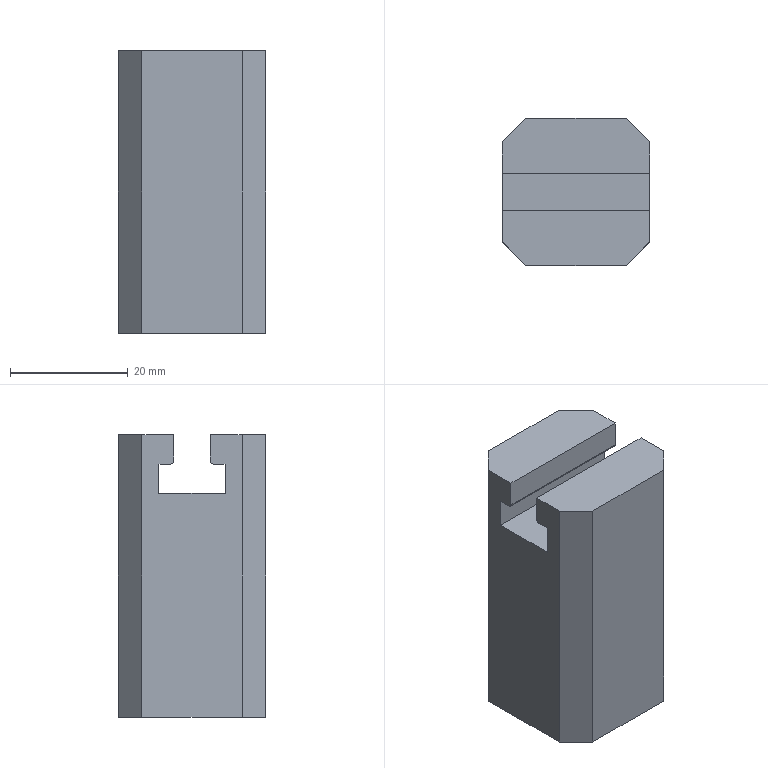Part | Creo | 1 solid | 153 faces | box 25 x 25 x 48 mm | volume 24480 mm3 | other 91 | plane 51 | cylinder 9 | cone 2 | commonest cylinder face diameters 1 x2 1.208 x2 8.499 x2 8.5 x2 19.045 x1